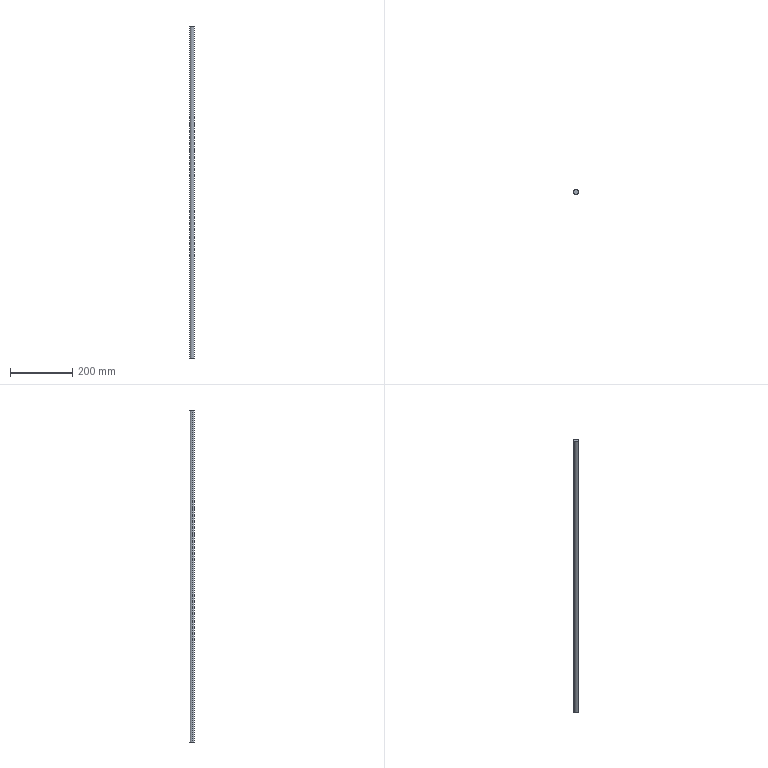Part | STEP file | 1 solid | 4 faces | box 16 x 16 x 1069 mm | volume 214935 mm3 | cylinder 2 | plane 2 | commonest cylinder face diameters 16 x2
STEP:
#1=CARTESIAN_POINT('',(0.,0.,0.));
#2=DIRECTION('',(0.,0.,1.));
#3=DIRECTION('',(1.,0.,0.));
#4=AXIS2_PLACEMENT_3D('',#1,#2,#3);
#5=CARTESIAN_POINT('',(8.,0.,534.5));
#6=VERTEX_POINT('',#5);
#7=CARTESIAN_POINT('',(-8.,0.,534.5));
#8=VERTEX_POINT('',#7);
#9=CARTESIAN_POINT('',(0.,0.,534.5));
#10=DIRECTION('',(0.,0.,1.));
#11=DIRECTION('',(1.,0.,0.));
#12=AXIS2_PLACEMENT_3D('',#9,#10,#11);
#13=CIRCLE('',#12,8.);
#14=CARTESIAN_POINT('',(0.,0.,534.5));
#15=DIRECTION('',(0.,0.,-1.));
#16=DIRECTION('',(-1.,0.,0.));
#17=AXIS2_PLACEMENT_3D('',#14,#15,#16);
#18=CYLINDRICAL_SURFACE('',#17,8.);
#19=CARTESIAN_POINT('',(3.142,0.));
#20=DIRECTION('',(-1.,0.));
#21=VECTOR('',#20,1.);
#22=LINE('',#19,#21);
#23=(GEOMETRIC_REPRESENTATION_CONTEXT(2)PARAMETRIC_REPRESENTATION_CONTEXT()REPRESENTATION_CONTEXT('',''));
#24=DEFINITIONAL_REPRESENTATION('',(#22),#23);
#25=PCURVE('',#18,#24);
#26=CARTESIAN_POINT('',(0.,0.,534.5));
#27=DIRECTION('',(0.,0.,1.));
#28=DIRECTION('',(1.,0.,0.));
#29=AXIS2_PLACEMENT_3D('',#26,#27,#28);
#30=PLANE('',#29);
#31=CARTESIAN_POINT('',(0.,0.));
#32=DIRECTION('',(1.,0.));
#33=AXIS2_PLACEMENT_2D('',#31,#32);
#34=CIRCLE('',#33,8.);
#35=(GEOMETRIC_REPRESENTATION_CONTEXT(2)PARAMETRIC_REPRESENTATION_CONTEXT()REPRESENTATION_CONTEXT('',''));
#36=DEFINITIONAL_REPRESENTATION('',(#34),#35);
#37=PCURVE('',#30,#36);
#38=SURFACE_CURVE('',#13,(#25,#37),.PCURVE_S1.);
#39=EDGE_CURVE('',#6,#8,#38,.T.);
#40=ORIENTED_EDGE('',*,*,#39,.F.);
#41=CARTESIAN_POINT('',(8.,0.,-534.5));
#42=VERTEX_POINT('',#41);
#43=CARTESIAN_POINT('',(8.,0.,534.5));
#44=DIRECTION('',(0.,0.,-1.));
#45=VECTOR('',#44,1.);
#46=LINE('',#43,#45);
#47=CARTESIAN_POINT('',(3.142,0.));
#48=DIRECTION('',(0.,1.));
#49=VECTOR('',#48,1.);
#50=LINE('',#47,#49);
#51=(GEOMETRIC_REPRESENTATION_CONTEXT(2)PARAMETRIC_REPRESENTATION_CONTEXT()REPRESENTATION_CONTEXT('',''));
#52=DEFINITIONAL_REPRESENTATION('',(#50),#51);
#53=PCURVE('',#18,#52);
#54=CARTESIAN_POINT('',(0.,0.,534.5));
#55=DIRECTION('',(0.,0.,-1.));
#56=DIRECTION('',(-1.,0.,0.));
#57=AXIS2_PLACEMENT_3D('',#54,#55,#56);
#58=CYLINDRICAL_SURFACE('',#57,8.);
#59=CARTESIAN_POINT('',(3.142,0.));
#60=DIRECTION('',(0.,1.));
#61=VECTOR('',#60,1.);
#62=LINE('',#59,#61);
#63=(GEOMETRIC_REPRESENTATION_CONTEXT(2)PARAMETRIC_REPRESENTATION_CONTEXT()REPRESENTATION_CONTEXT('',''));
#64=DEFINITIONAL_REPRESENTATION('',(#62),#63);
#65=PCURVE('',#58,#64);
#66=SURFACE_CURVE('',#46,(#53,#65),.PCURVE_S1.);
#67=EDGE_CURVE('',#6,#42,#66,.T.);
#68=ORIENTED_EDGE('',*,*,#67,.T.);
#69=CARTESIAN_POINT('',(-8.,0.,-534.5));
#70=VERTEX_POINT('',#69);
#71=CARTESIAN_POINT('',(0.,0.,-534.5));
#72=DIRECTION('',(0.,0.,1.));
#73=DIRECTION('',(1.,0.,0.));
#74=AXIS2_PLACEMENT_3D('',#71,#72,#73);
#75=CIRCLE('',#74,8.);
#76=CARTESIAN_POINT('',(3.142,1069.));
#77=DIRECTION('',(-1.,0.));
#78=VECTOR('',#77,1.);
#79=LINE('',#76,#78);
#80=(GEOMETRIC_REPRESENTATION_CONTEXT(2)PARAMETRIC_REPRESENTATION_CONTEXT()REPRESENTATION_CONTEXT('',''));
#81=DEFINITIONAL_REPRESENTATION('',(#79),#80);
#82=PCURVE('',#18,#81);
#83=CARTESIAN_POINT('',(0.,0.,-534.5));
#84=DIRECTION('',(0.,0.,1.));
#85=DIRECTION('',(1.,0.,0.));
#86=AXIS2_PLACEMENT_3D('',#83,#84,#85);
#87=PLANE('',#86);
#88=CARTESIAN_POINT('',(0.,0.));
#89=DIRECTION('',(1.,0.));
#90=AXIS2_PLACEMENT_2D('',#88,#89);
#91=CIRCLE('',#90,8.);
#92=(GEOMETRIC_REPRESENTATION_CONTEXT(2)PARAMETRIC_REPRESENTATION_CONTEXT()REPRESENTATION_CONTEXT('',''));
#93=DEFINITIONAL_REPRESENTATION('',(#91),#92);
#94=PCURVE('',#87,#93);
#95=SURFACE_CURVE('',#75,(#82,#94),.PCURVE_S1.);
#96=EDGE_CURVE('',#42,#70,#95,.T.);
#97=ORIENTED_EDGE('',*,*,#96,.T.);
#98=CARTESIAN_POINT('',(-8.,0.,534.5));
#99=DIRECTION('',(0.,0.,-1.));
#100=VECTOR('',#99,1.);
#101=LINE('',#98,#100);
#102=CARTESIAN_POINT('',(0.,0.));
#103=DIRECTION('',(0.,1.));
#104=VECTOR('',#103,1.);
#105=LINE('',#102,#104);
#106=(GEOMETRIC_REPRESENTATION_CONTEXT(2)PARAMETRIC_REPRESENTATION_CONTEXT()REPRESENTATION_CONTEXT('',''));
#107=DEFINITIONAL_REPRESENTATION('',(#105),#106);
#108=PCURVE('',#18,#107);
#109=CARTESIAN_POINT('',(6.283,0.));
#110=DIRECTION('',(0.,1.));
#111=VECTOR('',#110,1.);
#112=LINE('',#109,#111);
#113=(GEOMETRIC_REPRESENTATION_CONTEXT(2)PARAMETRIC_REPRESENTATION_CONTEXT()REPRESENTATION_CONTEXT('',''));
#114=DEFINITIONAL_REPRESENTATION('',(#112),#113);
#115=PCURVE('',#58,#114);
#116=SURFACE_CURVE('',#101,(#108,#115),.PCURVE_S1.);
#117=EDGE_CURVE('',#8,#70,#116,.T.);
#118=ORIENTED_EDGE('',*,*,#117,.F.);
#119=EDGE_LOOP('',(#40,#68,#97,#118));
#120=FACE_BOUND('',#119,.T.);
#121=ADVANCED_FACE('',(#120),#18,.T.);
#122=ORIENTED_EDGE('',*,*,#67,.F.);
#123=CARTESIAN_POINT('',(0.,0.,534.5));
#124=DIRECTION('',(0.,0.,1.));
#125=DIRECTION('',(1.,0.,0.));
#126=AXIS2_PLACEMENT_3D('',#123,#124,#125);
#127=CIRCLE('',#126,8.);
#128=CARTESIAN_POINT('',(9.425,0.));
#129=DIRECTION('',(-1.,0.));
#130=VECTOR('',#129,1.);
#131=LINE('',#128,#130);
#132=(GEOMETRIC_REPRESENTATION_CONTEXT(2)PARAMETRIC_REPRESENTATION_CONTEXT()REPRESENTATION_CONTEXT('',''));
#133=DEFINITIONAL_REPRESENTATION('',(#131),#132);
#134=PCURVE('',#58,#133);
#135=CARTESIAN_POINT('',(0.,0.));
#136=DIRECTION('',(1.,0.));
#137=AXIS2_PLACEMENT_2D('',#135,#136);
#138=CIRCLE('',#137,8.);
#139=(GEOMETRIC_REPRESENTATION_CONTEXT(2)PARAMETRIC_REPRESENTATION_CONTEXT()REPRESENTATION_CONTEXT('',''));
#140=DEFINITIONAL_REPRESENTATION('',(#138),#139);
#141=PCURVE('',#30,#140);
#142=SURFACE_CURVE('',#127,(#134,#141),.PCURVE_S1.);
#143=EDGE_CURVE('',#8,#6,#142,.T.);
#144=ORIENTED_EDGE('',*,*,#143,.F.);
#145=ORIENTED_EDGE('',*,*,#117,.T.);
#146=CARTESIAN_POINT('',(0.,0.,-534.5));
#147=DIRECTION('',(0.,0.,1.));
#148=DIRECTION('',(1.,0.,0.));
#149=AXIS2_PLACEMENT_3D('',#146,#147,#148);
#150=CIRCLE('',#149,8.);
#151=CARTESIAN_POINT('',(9.425,1069.));
#152=DIRECTION('',(-1.,0.));
#153=VECTOR('',#152,1.);
#154=LINE('',#151,#153);
#155=(GEOMETRIC_REPRESENTATION_CONTEXT(2)PARAMETRIC_REPRESENTATION_CONTEXT()REPRESENTATION_CONTEXT('',''));
#156=DEFINITIONAL_REPRESENTATION('',(#154),#155);
#157=PCURVE('',#58,#156);
#158=CARTESIAN_POINT('',(0.,0.));
#159=DIRECTION('',(1.,0.));
#160=AXIS2_PLACEMENT_2D('',#158,#159);
#161=CIRCLE('',#160,8.);
#162=(GEOMETRIC_REPRESENTATION_CONTEXT(2)PARAMETRIC_REPRESENTATION_CONTEXT()REPRESENTATION_CONTEXT('',''));
#163=DEFINITIONAL_REPRESENTATION('',(#161),#162);
#164=PCURVE('',#87,#163);
#165=SURFACE_CURVE('',#150,(#157,#164),.PCURVE_S1.);
#166=EDGE_CURVE('',#70,#42,#165,.T.);
#167=ORIENTED_EDGE('',*,*,#166,.T.);
#168=EDGE_LOOP('',(#122,#144,#145,#167));
#169=FACE_BOUND('',#168,.T.);
#170=ADVANCED_FACE('',(#169),#58,.T.);
#171=ORIENTED_EDGE('',*,*,#143,.T.);
#172=ORIENTED_EDGE('',*,*,#39,.T.);
#173=EDGE_LOOP('',(#171,#172));
#174=FACE_BOUND('',#173,.T.);
#175=ADVANCED_FACE('',(#174),#30,.T.);
#176=ORIENTED_EDGE('',*,*,#166,.F.);
#177=ORIENTED_EDGE('',*,*,#96,.F.);
#178=EDGE_LOOP('',(#176,#177));
#179=FACE_BOUND('',#178,.T.);
#180=ADVANCED_FACE('',(#179),#87,.F.);
#181=CLOSED_SHELL('',(#121,#170,#175,#180));
#182=MANIFOLD_SOLID_BREP('',#181);
#183=(LENGTH_UNIT()NAMED_UNIT(*)SI_UNIT(.MILLI.,.METRE.));
#184=UNCERTAINTY_MEASURE_WITH_UNIT(LENGTH_MEASURE(0.0000001),#183,'','');
#185=(NAMED_UNIT(*)PLANE_ANGLE_UNIT()SI_UNIT($,.RADIAN.));
#186=(NAMED_UNIT(*)SI_UNIT($,.STERADIAN.)SOLID_ANGLE_UNIT());
#187=(GEOMETRIC_REPRESENTATION_CONTEXT(3)GLOBAL_UNCERTAINTY_ASSIGNED_CONTEXT((#184))GLOBAL_UNIT_ASSIGNED_CONTEXT((#183,#185,#186))REPRESENTATION_CONTEXT('',''));
#188=ADVANCED_BREP_SHAPE_REPRESENTATION('',(#4,#182),#187);